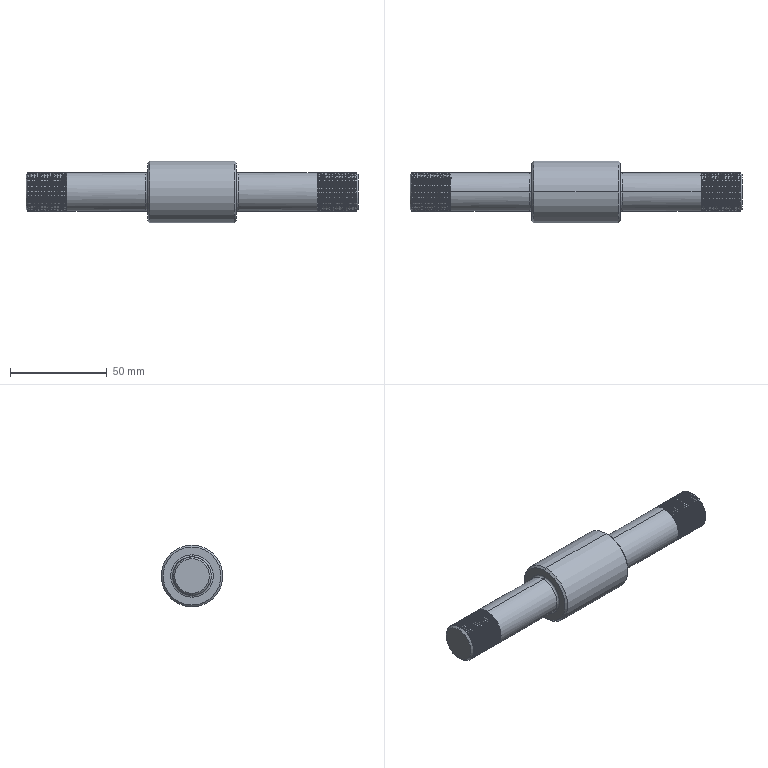Part | STEP file | Hinge pin stepped shaft 2 | 1 solid | 232 faces | box 172 x 32 x 32 mm | volume 76081 mm3 | cylinder 206 | cone 8 | plane 8 | spline 6 | torus 4 | commonest cylinder face diameters 20 x204 32 x2